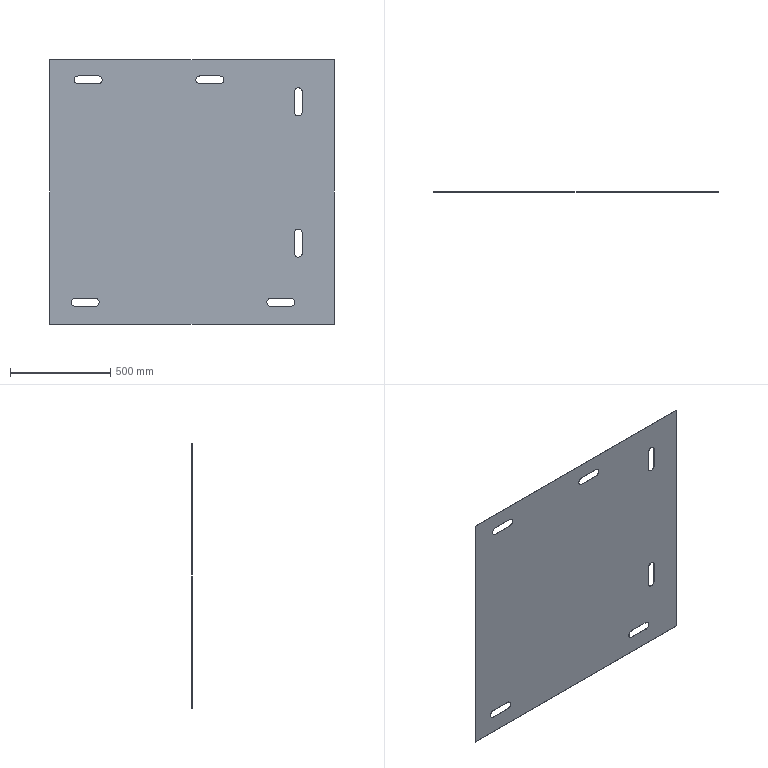Part | NX | features 切除-拉伸1 2 | 1 solid | 32 faces | box 1420 x 2 x 1320 mm | volume 3685720 mm3 | plane 18 | cylinder 14 | commonest cylinder face diameters 40 x14
STEP:
#1=CARTESIAN_POINT('',(622.78,-600.,-93.003));
#2=VERTEX_POINT('',#1);
#3=CARTESIAN_POINT('',(722.78,-600.,-93.003));
#4=VERTEX_POINT('',#3);
#5=CARTESIAN_POINT('',(622.78,-600.,-93.003));
#6=DIRECTION('',(1.,0.,0.));
#7=VECTOR('',#6,1000.);
#8=LINE('',#5,#7);
#9=EDGE_CURVE('',#2,#4,#8,.T.);
#10=ORIENTED_EDGE('',*,*,#9,.T.);
#11=CARTESIAN_POINT('',(722.78,-602.,-93.003));
#12=VERTEX_POINT('',#11);
#13=CARTESIAN_POINT('',(722.78,-602.,-93.003));
#14=DIRECTION('',(0.,1.,0.));
#15=VECTOR('',#14,1000.);
#16=LINE('',#13,#15);
#17=EDGE_CURVE('',#12,#4,#16,.T.);
#18=ORIENTED_EDGE('',*,*,#17,.F.);
#19=CARTESIAN_POINT('',(622.78,-602.,-93.003));
#20=VERTEX_POINT('',#19);
#21=CARTESIAN_POINT('',(622.78,-602.,-93.003));
#22=DIRECTION('',(1.,0.,0.));
#23=VECTOR('',#22,1000.);
#24=LINE('',#21,#23);
#25=EDGE_CURVE('',#20,#12,#24,.T.);
#26=ORIENTED_EDGE('',*,*,#25,.F.);
#27=CARTESIAN_POINT('',(622.78,-602.,-93.003));
#28=DIRECTION('',(0.,1.,0.));
#29=VECTOR('',#28,1000.);
#30=LINE('',#27,#29);
#31=EDGE_CURVE('',#20,#2,#30,.T.);
#32=ORIENTED_EDGE('',*,*,#31,.T.);
#33=EDGE_LOOP('',(#10,#18,#26,#32));
#34=FACE_BOUND('',#33,.T.);
#35=CARTESIAN_POINT('',(622.78,-602.,-93.003));
#36=DIRECTION('',(0.,0.,1.));
#37=DIRECTION('',(1.,0.,0.));
#38=AXIS2_PLACEMENT_3D('',#35,#36,#37);
#39=PLANE('',#38);
#40=ADVANCED_FACE('',(#34),#39,.F.);
#41=CARTESIAN_POINT('',(722.78,-600.,-133.003));
#42=VERTEX_POINT('',#41);
#43=CARTESIAN_POINT('',(722.78,-600.,-113.003));
#44=DIRECTION('',(0.,1.,0.));
#45=DIRECTION('',(0.,0.,1.));
#46=AXIS2_PLACEMENT_3D('',#43,#44,#45);
#47=CIRCLE('',#46,20.);
#48=EDGE_CURVE('',#4,#42,#47,.T.);
#49=ORIENTED_EDGE('',*,*,#48,.T.);
#50=CARTESIAN_POINT('',(722.78,-602.,-133.003));
#51=VERTEX_POINT('',#50);
#52=CARTESIAN_POINT('',(722.78,-602.,-133.003));
#53=DIRECTION('',(0.,1.,0.));
#54=VECTOR('',#53,1000.);
#55=LINE('',#52,#54);
#56=EDGE_CURVE('',#51,#42,#55,.T.);
#57=ORIENTED_EDGE('',*,*,#56,.F.);
#58=CARTESIAN_POINT('',(722.78,-602.,-113.003));
#59=DIRECTION('',(0.,1.,0.));
#60=DIRECTION('',(0.,0.,1.));
#61=AXIS2_PLACEMENT_3D('',#58,#59,#60);
#62=CIRCLE('',#61,20.);
#63=EDGE_CURVE('',#12,#51,#62,.T.);
#64=ORIENTED_EDGE('',*,*,#63,.F.);
#65=ORIENTED_EDGE('',*,*,#17,.T.);
#66=EDGE_LOOP('',(#49,#57,#64,#65));
#67=FACE_BOUND('',#66,.T.);
#68=CARTESIAN_POINT('',(722.78,-602.,-113.003));
#69=DIRECTION('',(0.,1.,0.));
#70=DIRECTION('',(0.,0.,1.));
#71=AXIS2_PLACEMENT_3D('',#68,#69,#70);
#72=CYLINDRICAL_SURFACE('',#71,20.);
#73=ADVANCED_FACE('',(#67),#72,.F.);
#74=CARTESIAN_POINT('',(622.78,-600.,-133.003));
#75=VERTEX_POINT('',#74);
#76=CARTESIAN_POINT('',(622.78,-600.,-133.003));
#77=DIRECTION('',(-1.,0.,0.));
#78=VECTOR('',#77,1000.);
#79=LINE('',#76,#78);
#80=EDGE_CURVE('',#42,#75,#79,.T.);
#81=ORIENTED_EDGE('',*,*,#80,.T.);
#82=CARTESIAN_POINT('',(622.78,-602.,-133.003));
#83=VERTEX_POINT('',#82);
#84=CARTESIAN_POINT('',(622.78,-602.,-133.003));
#85=DIRECTION('',(0.,1.,0.));
#86=VECTOR('',#85,1000.);
#87=LINE('',#84,#86);
#88=EDGE_CURVE('',#83,#75,#87,.T.);
#89=ORIENTED_EDGE('',*,*,#88,.F.);
#90=CARTESIAN_POINT('',(622.78,-602.,-133.003));
#91=DIRECTION('',(-1.,0.,0.));
#92=VECTOR('',#91,1000.);
#93=LINE('',#90,#92);
#94=EDGE_CURVE('',#51,#83,#93,.T.);
#95=ORIENTED_EDGE('',*,*,#94,.F.);
#96=ORIENTED_EDGE('',*,*,#56,.T.);
#97=EDGE_LOOP('',(#81,#89,#95,#96));
#98=FACE_BOUND('',#97,.T.);
#99=CARTESIAN_POINT('',(622.78,-602.,-133.003));
#100=DIRECTION('',(0.,0.,-1.));
#101=DIRECTION('',(-1.,0.,0.));
#102=AXIS2_PLACEMENT_3D('',#99,#100,#101);
#103=PLANE('',#102);
#104=ADVANCED_FACE('',(#98),#103,.F.);
#105=CARTESIAN_POINT('',(622.78,-600.,-113.003));
#106=DIRECTION('',(0.,1.,0.));
#107=DIRECTION('',(0.,0.,1.));
#108=AXIS2_PLACEMENT_3D('',#105,#106,#107);
#109=CIRCLE('',#108,20.);
#110=EDGE_CURVE('',#75,#2,#109,.T.);
#111=ORIENTED_EDGE('',*,*,#110,.T.);
#112=ORIENTED_EDGE('',*,*,#31,.F.);
#113=CARTESIAN_POINT('',(622.78,-602.,-113.003));
#114=DIRECTION('',(0.,1.,0.));
#115=DIRECTION('',(0.,0.,1.));
#116=AXIS2_PLACEMENT_3D('',#113,#114,#115);
#117=CIRCLE('',#116,20.);
#118=EDGE_CURVE('',#83,#20,#117,.T.);
#119=ORIENTED_EDGE('',*,*,#118,.F.);
#120=ORIENTED_EDGE('',*,*,#88,.T.);
#121=EDGE_LOOP('',(#111,#112,#119,#120));
#122=FACE_BOUND('',#121,.T.);
#123=CARTESIAN_POINT('',(622.78,-602.,-113.003));
#124=DIRECTION('',(0.,1.,0.));
#125=DIRECTION('',(0.,0.,1.));
#126=AXIS2_PLACEMENT_3D('',#123,#124,#125);
#127=CYLINDRICAL_SURFACE('',#126,20.);
#128=ADVANCED_FACE('',(#122),#127,.F.);
#129=CARTESIAN_POINT('',(-0.6402,-600.,-1204.113));
#130=VERTEX_POINT('',#129);
#131=CARTESIAN_POINT('',(99.36,-600.,-1204.113));
#132=VERTEX_POINT('',#131);
#133=CARTESIAN_POINT('',(-0.6402,-600.,-1204.113));
#134=DIRECTION('',(1.,0.,0.));
#135=VECTOR('',#134,1000.);
#136=LINE('',#133,#135);
#137=EDGE_CURVE('',#130,#132,#136,.T.);
#138=ORIENTED_EDGE('',*,*,#137,.T.);
#139=CARTESIAN_POINT('',(99.36,-602.,-1204.113));
#140=VERTEX_POINT('',#139);
#141=CARTESIAN_POINT('',(99.36,-602.,-1204.113));
#142=DIRECTION('',(0.,1.,0.));
#143=VECTOR('',#142,1000.);
#144=LINE('',#141,#143);
#145=EDGE_CURVE('',#140,#132,#144,.T.);
#146=ORIENTED_EDGE('',*,*,#145,.F.);
#147=CARTESIAN_POINT('',(-0.6402,-602.,-1204.113));
#148=VERTEX_POINT('',#147);
#149=CARTESIAN_POINT('',(-0.6402,-602.,-1204.113));
#150=DIRECTION('',(1.,0.,0.));
#151=VECTOR('',#150,1000.);
#152=LINE('',#149,#151);
#153=EDGE_CURVE('',#148,#140,#152,.T.);
#154=ORIENTED_EDGE('',*,*,#153,.F.);
#155=CARTESIAN_POINT('',(-0.6402,-602.,-1204.113));
#156=DIRECTION('',(0.,1.,0.));
#157=VECTOR('',#156,1000.);
#158=LINE('',#155,#157);
#159=EDGE_CURVE('',#148,#130,#158,.T.);
#160=ORIENTED_EDGE('',*,*,#159,.T.);
#161=EDGE_LOOP('',(#138,#146,#154,#160));
#162=FACE_BOUND('',#161,.T.);
#163=CARTESIAN_POINT('',(-0.6402,-602.,-1204.113));
#164=DIRECTION('',(0.,0.,1.));
#165=DIRECTION('',(1.,0.,0.));
#166=AXIS2_PLACEMENT_3D('',#163,#164,#165);
#167=PLANE('',#166);
#168=ADVANCED_FACE('',(#162),#167,.F.);
#169=CARTESIAN_POINT('',(99.36,-600.,-1244.113));
#170=VERTEX_POINT('',#169);
#171=CARTESIAN_POINT('',(99.36,-600.,-1224.113));
#172=DIRECTION('',(0.,1.,0.));
#173=DIRECTION('',(0.,0.,1.));
#174=AXIS2_PLACEMENT_3D('',#171,#172,#173);
#175=CIRCLE('',#174,20.);
#176=EDGE_CURVE('',#132,#170,#175,.T.);
#177=ORIENTED_EDGE('',*,*,#176,.T.);
#178=CARTESIAN_POINT('',(99.36,-602.,-1244.113));
#179=VERTEX_POINT('',#178);
#180=CARTESIAN_POINT('',(99.36,-602.,-1244.113));
#181=DIRECTION('',(0.,1.,0.));
#182=VECTOR('',#181,1000.);
#183=LINE('',#180,#182);
#184=EDGE_CURVE('',#179,#170,#183,.T.);
#185=ORIENTED_EDGE('',*,*,#184,.F.);
#186=CARTESIAN_POINT('',(99.36,-602.,-1224.113));
#187=DIRECTION('',(0.,1.,0.));
#188=DIRECTION('',(0.,0.,1.));
#189=AXIS2_PLACEMENT_3D('',#186,#187,#188);
#190=CIRCLE('',#189,20.);
#191=EDGE_CURVE('',#140,#179,#190,.T.);
#192=ORIENTED_EDGE('',*,*,#191,.F.);
#193=ORIENTED_EDGE('',*,*,#145,.T.);
#194=EDGE_LOOP('',(#177,#185,#192,#193));
#195=FACE_BOUND('',#194,.T.);
#196=CARTESIAN_POINT('',(99.36,-602.,-1224.113));
#197=DIRECTION('',(0.,1.,0.));
#198=DIRECTION('',(0.,0.,1.));
#199=AXIS2_PLACEMENT_3D('',#196,#197,#198);
#200=CYLINDRICAL_SURFACE('',#199,20.);
#201=ADVANCED_FACE('',(#195),#200,.F.);
#202=CARTESIAN_POINT('',(-0.6402,-600.,-1244.113));
#203=VERTEX_POINT('',#202);
#204=CARTESIAN_POINT('',(-0.6402,-600.,-1244.113));
#205=DIRECTION('',(-1.,0.,0.));
#206=VECTOR('',#205,1000.);
#207=LINE('',#204,#206);
#208=EDGE_CURVE('',#170,#203,#207,.T.);
#209=ORIENTED_EDGE('',*,*,#208,.T.);
#210=CARTESIAN_POINT('',(-0.6402,-602.,-1244.113));
#211=VERTEX_POINT('',#210);
#212=CARTESIAN_POINT('',(-0.6402,-602.,-1244.113));
#213=DIRECTION('',(0.,1.,0.));
#214=VECTOR('',#213,1000.);
#215=LINE('',#212,#214);
#216=EDGE_CURVE('',#211,#203,#215,.T.);
#217=ORIENTED_EDGE('',*,*,#216,.F.);
#218=CARTESIAN_POINT('',(-0.6402,-602.,-1244.113));
#219=DIRECTION('',(-1.,0.,0.));
#220=VECTOR('',#219,1000.);
#221=LINE('',#218,#220);
#222=EDGE_CURVE('',#179,#211,#221,.T.);
#223=ORIENTED_EDGE('',*,*,#222,.F.);
#224=ORIENTED_EDGE('',*,*,#184,.T.);
#225=EDGE_LOOP('',(#209,#217,#223,#224));
#226=FACE_BOUND('',#225,.T.);
#227=CARTESIAN_POINT('',(-0.6402,-602.,-1244.113));
#228=DIRECTION('',(0.,0.,-1.));
#229=DIRECTION('',(-1.,0.,0.));
#230=AXIS2_PLACEMENT_3D('',#227,#228,#229);
#231=PLANE('',#230);
#232=ADVANCED_FACE('',(#226),#231,.F.);
#233=CARTESIAN_POINT('',(-0.6402,-600.,-1224.113));
#234=DIRECTION('',(0.,1.,0.));
#235=DIRECTION('',(0.,0.,1.));
#236=AXIS2_PLACEMENT_3D('',#233,#234,#235);
#237=CIRCLE('',#236,20.);
#238=EDGE_CURVE('',#203,#130,#237,.T.);
#239=ORIENTED_EDGE('',*,*,#238,.T.);
#240=ORIENTED_EDGE('',*,*,#159,.F.);
#241=CARTESIAN_POINT('',(-0.6402,-602.,-1224.113));
#242=DIRECTION('',(0.,1.,0.));
#243=DIRECTION('',(0.,0.,1.));
#244=AXIS2_PLACEMENT_3D('',#241,#242,#243);
#245=CIRCLE('',#244,20.);
#246=EDGE_CURVE('',#211,#148,#245,.T.);
#247=ORIENTED_EDGE('',*,*,#246,.F.);
#248=ORIENTED_EDGE('',*,*,#216,.T.);
#249=EDGE_LOOP('',(#239,#240,#247,#248));
#250=FACE_BOUND('',#249,.T.);
#251=CARTESIAN_POINT('',(-0.6402,-602.,-1224.113));
#252=DIRECTION('',(0.,1.,0.));
#253=DIRECTION('',(0.,0.,1.));
#254=AXIS2_PLACEMENT_3D('',#251,#252,#253);
#255=CYLINDRICAL_SURFACE('',#254,20.);
#256=ADVANCED_FACE('',(#250),#255,.F.);
#257=CARTESIAN_POINT('',(976.615,-600.,-1204.113));
#258=VERTEX_POINT('',#257);
#259=CARTESIAN_POINT('',(1076.615,-600.,-1204.113));
#260=VERTEX_POINT('',#259);
#261=CARTESIAN_POINT('',(976.615,-600.,-1204.113));
#262=DIRECTION('',(1.,0.,0.));
#263=VECTOR('',#262,1000.);
#264=LINE('',#261,#263);
#265=EDGE_CURVE('',#258,#260,#264,.T.);
#266=ORIENTED_EDGE('',*,*,#265,.T.);
#267=CARTESIAN_POINT('',(1076.615,-602.,-1204.113));
#268=VERTEX_POINT('',#267);
#269=CARTESIAN_POINT('',(1076.615,-602.,-1204.113));
#270=DIRECTION('',(0.,1.,0.));
#271=VECTOR('',#270,1000.);
#272=LINE('',#269,#271);
#273=EDGE_CURVE('',#268,#260,#272,.T.);
#274=ORIENTED_EDGE('',*,*,#273,.F.);
#275=CARTESIAN_POINT('',(976.615,-602.,-1204.113));
#276=VERTEX_POINT('',#275);
#277=CARTESIAN_POINT('',(976.615,-602.,-1204.113));
#278=DIRECTION('',(1.,0.,0.));
#279=VECTOR('',#278,1000.);
#280=LINE('',#277,#279);
#281=EDGE_CURVE('',#276,#268,#280,.T.);
#282=ORIENTED_EDGE('',*,*,#281,.F.);
#283=CARTESIAN_POINT('',(976.615,-602.,-1204.113));
#284=DIRECTION('',(0.,1.,0.));
#285=VECTOR('',#284,1000.);
#286=LINE('',#283,#285);
#287=EDGE_CURVE('',#276,#258,#286,.T.);
#288=ORIENTED_EDGE('',*,*,#287,.T.);
#289=EDGE_LOOP('',(#266,#274,#282,#288));
#290=FACE_BOUND('',#289,.T.);
#291=CARTESIAN_POINT('',(976.615,-602.,-1204.113));
#292=DIRECTION('',(0.,0.,1.));
#293=DIRECTION('',(1.,0.,0.));
#294=AXIS2_PLACEMENT_3D('',#291,#292,#293);
#295=PLANE('',#294);
#296=ADVANCED_FACE('',(#290),#295,.F.);
#297=CARTESIAN_POINT('',(1076.615,-600.,-1244.113));
#298=VERTEX_POINT('',#297);
#299=CARTESIAN_POINT('',(1076.615,-600.,-1224.113));
#300=DIRECTION('',(0.,1.,0.));
#301=DIRECTION('',(0.,0.,1.));
#302=AXIS2_PLACEMENT_3D('',#299,#300,#301);
#303=CIRCLE('',#302,20.);
#304=EDGE_CURVE('',#260,#298,#303,.T.);
#305=ORIENTED_EDGE('',*,*,#304,.T.);
#306=CARTESIAN_POINT('',(1076.615,-602.,-1244.113));
#307=VERTEX_POINT('',#306);
#308=CARTESIAN_POINT('',(1076.615,-602.,-1244.113));
#309=DIRECTION('',(0.,1.,0.));
#310=VECTOR('',#309,1000.);
#311=LINE('',#308,#310);
#312=EDGE_CURVE('',#307,#298,#311,.T.);
#313=ORIENTED_EDGE('',*,*,#312,.F.);
#314=CARTESIAN_POINT('',(1076.615,-602.,-1224.113));
#315=DIRECTION('',(0.,1.,0.));
#316=DIRECTION('',(0.,0.,1.));
#317=AXIS2_PLACEMENT_3D('',#314,#315,#316);
#318=CIRCLE('',#317,20.);
#319=EDGE_CURVE('',#268,#307,#318,.T.);
#320=ORIENTED_EDGE('',*,*,#319,.F.);
#321=ORIENTED_EDGE('',*,*,#273,.T.);
#322=EDGE_LOOP('',(#305,#313,#320,#321));
#323=FACE_BOUND('',#322,.T.);
#324=CARTESIAN_POINT('',(1076.615,-602.,-1224.113));
#325=DIRECTION('',(0.,1.,0.));
#326=DIRECTION('',(0.,0.,1.));
#327=AXIS2_PLACEMENT_3D('',#324,#325,#326);
#328=CYLINDRICAL_SURFACE('',#327,20.);
#329=ADVANCED_FACE('',(#323),#328,.F.);
#330=CARTESIAN_POINT('',(976.615,-600.,-1244.113));
#331=VERTEX_POINT('',#330);
#332=CARTESIAN_POINT('',(976.615,-600.,-1244.113));
#333=DIRECTION('',(-1.,0.,0.));
#334=VECTOR('',#333,1000.);
#335=LINE('',#332,#334);
#336=EDGE_CURVE('',#298,#331,#335,.T.);
#337=ORIENTED_EDGE('',*,*,#336,.T.);
#338=CARTESIAN_POINT('',(976.615,-602.,-1244.113));
#339=VERTEX_POINT('',#338);
#340=CARTESIAN_POINT('',(976.615,-602.,-1244.113));
#341=DIRECTION('',(0.,1.,0.));
#342=VECTOR('',#341,1000.);
#343=LINE('',#340,#342);
#344=EDGE_CURVE('',#339,#331,#343,.T.);
#345=ORIENTED_EDGE('',*,*,#344,.F.);
#346=CARTESIAN_POINT('',(976.615,-602.,-1244.113));
#347=DIRECTION('',(-1.,0.,0.));
#348=VECTOR('',#347,1000.);
#349=LINE('',#346,#348);
#350=EDGE_CURVE('',#307,#339,#349,.T.);
#351=ORIENTED_EDGE('',*,*,#350,.F.);
#352=ORIENTED_EDGE('',*,*,#312,.T.);
#353=EDGE_LOOP('',(#337,#345,#351,#352));
#354=FACE_BOUND('',#353,.T.);
#355=CARTESIAN_POINT('',(976.615,-602.,-1244.113));
#356=DIRECTION('',(0.,0.,-1.));
#357=DIRECTION('',(-1.,0.,0.));
#358=AXIS2_PLACEMENT_3D('',#355,#356,#357);
#359=PLANE('',#358);
#360=ADVANCED_FACE('',(#354),#359,.F.);
#361=CARTESIAN_POINT('',(976.615,-600.,-1224.113));
#362=DIRECTION('',(0.,1.,0.));
#363=DIRECTION('',(0.,0.,1.));
#364=AXIS2_PLACEMENT_3D('',#361,#362,#363);
#365=CIRCLE('',#364,20.);
#366=EDGE_CURVE('',#331,#258,#365,.T.);
#367=ORIENTED_EDGE('',*,*,#366,.T.);
#368=ORIENTED_EDGE('',*,*,#287,.F.);
#369=CARTESIAN_POINT('',(976.615,-602.,-1224.113));
#370=DIRECTION('',(0.,1.,0.));
#371=DIRECTION('',(0.,0.,1.));
#372=AXIS2_PLACEMENT_3D('',#369,#370,#371);
#373=CIRCLE('',#372,20.);
#374=EDGE_CURVE('',#339,#276,#373,.T.);
#375=ORIENTED_EDGE('',*,*,#374,.F.);
#376=ORIENTED_EDGE('',*,*,#344,.T.);
#377=EDGE_LOOP('',(#367,#368,#375,#376));
#378=FACE_BOUND('',#377,.T.);
#379=CARTESIAN_POINT('',(976.615,-602.,-1224.113));
#380=DIRECTION('',(0.,1.,0.));
#381=DIRECTION('',(0.,0.,1.));
#382=AXIS2_PLACEMENT_3D('',#379,#380,#381);
#383=CYLINDRICAL_SURFACE('',#382,20.);
#384=ADVANCED_FACE('',(#378),#383,.F.);
#385=CARTESIAN_POINT('',(1133.771,-600.,-878.167));
#386=VERTEX_POINT('',#385);
#387=CARTESIAN_POINT('',(1133.771,-600.,-978.167));
#388=VERTEX_POINT('',#387);
#389=CARTESIAN_POINT('',(1133.771,-600.,-878.167));
#390=DIRECTION('',(0.,0.,-1.));
#391=VECTOR('',#390,1000.);
#392=LINE('',#389,#391);
#393=EDGE_CURVE('',#386,#388,#392,.T.);
#394=ORIENTED_EDGE('',*,*,#393,.T.);
#395=CARTESIAN_POINT('',(1133.771,-602.,-978.167));
#396=VERTEX_POINT('',#395);
#397=CARTESIAN_POINT('',(1133.771,-602.,-978.167));
#398=DIRECTION('',(0.,1.,0.));
#399=VECTOR('',#398,1000.);
#400=LINE('',#397,#399);
#401=EDGE_CURVE('',#396,#388,#400,.T.);
#402=ORIENTED_EDGE('',*,*,#401,.F.);
#403=CARTESIAN_POINT('',(1133.771,-602.,-878.167));
#404=VERTEX_POINT('',#403);
#405=CARTESIAN_POINT('',(1133.771,-602.,-878.167));
#406=DIRECTION('',(0.,0.,-1.));
#407=VECTOR('',#406,1000.);
#408=LINE('',#405,#407);
#409=EDGE_CURVE('',#404,#396,#408,.T.);
#410=ORIENTED_EDGE('',*,*,#409,.F.);
#411=CARTESIAN_POINT('',(1133.771,-602.,-878.167));
#412=DIRECTION('',(0.,1.,0.));
#413=VECTOR('',#412,1000.);
#414=LINE('',#411,#413);
#415=EDGE_CURVE('',#404,#386,#414,.T.);
#416=ORIENTED_EDGE('',*,*,#415,.T.);
#417=EDGE_LOOP('',(#394,#402,#410,#416));
#418=FACE_BOUND('',#417,.T.);
#419=CARTESIAN_POINT('',(1133.771,-602.,-878.167));
#420=DIRECTION('',(1.,0.,0.));
#421=DIRECTION('',(0.,0.,-1.));
#422=AXIS2_PLACEMENT_3D('',#419,#420,#421);
#423=PLANE('',#422);
#424=ADVANCED_FACE('',(#418),#423,.F.);
#425=CARTESIAN_POINT('',(1093.771,-600.,-978.167));
#426=VERTEX_POINT('',#425);
#427=CARTESIAN_POINT('',(1113.771,-600.,-978.167));
#428=DIRECTION('',(0.,1.,0.));
#429=DIRECTION('',(0.,0.,1.));
#430=AXIS2_PLACEMENT_3D('',#427,#428,#429);
#431=CIRCLE('',#430,20.);
#432=EDGE_CURVE('',#388,#426,#431,.T.);
#433=ORIENTED_EDGE('',*,*,#432,.T.);
#434=CARTESIAN_POINT('',(1093.771,-602.,-978.167));
#435=VERTEX_POINT('',#434);
#436=CARTESIAN_POINT('',(1093.771,-602.,-978.167));
#437=DIRECTION('',(0.,1.,0.));
#438=VECTOR('',#437,1000.);
#439=LINE('',#436,#438);
#440=EDGE_CURVE('',#435,#426,#439,.T.);
#441=ORIENTED_EDGE('',*,*,#440,.F.);
#442=CARTESIAN_POINT('',(1113.771,-602.,-978.167));
#443=DIRECTION('',(0.,1.,0.));
#444=DIRECTION('',(0.,0.,1.));
#445=AXIS2_PLACEMENT_3D('',#442,#443,#444);
#446=CIRCLE('',#445,20.);
#447=EDGE_CURVE('',#396,#435,#446,.T.);
#448=ORIENTED_EDGE('',*,*,#447,.F.);
#449=ORIENTED_EDGE('',*,*,#401,.T.);
#450=EDGE_LOOP('',(#433,#441,#448,#449));
#451=FACE_BOUND('',#450,.T.);
#452=CARTESIAN_POINT('',(1113.771,-602.,-978.167));
#453=DIRECTION('',(0.,1.,0.));
#454=DIRECTION('',(0.,0.,1.));
#455=AXIS2_PLACEMENT_3D('',#452,#453,#454);
#456=CYLINDRICAL_SURFACE('',#455,20.);
#457=ADVANCED_FACE('',(#451),#456,.F.);
#458=CARTESIAN_POINT('',(1093.771,-600.,-878.167));
#459=VERTEX_POINT('',#458);
#460=CARTESIAN_POINT('',(1093.771,-600.,-878.167));
#461=DIRECTION('',(0.,0.,1.));
#462=VECTOR('',#461,1000.);
#463=LINE('',#460,#462);
#464=EDGE_CURVE('',#426,#459,#463,.T.);
#465=ORIENTED_EDGE('',*,*,#464,.T.);
#466=CARTESIAN_POINT('',(1093.771,-602.,-878.167));
#467=VERTEX_POINT('',#466);
#468=CARTESIAN_POINT('',(1093.771,-602.,-878.167));
#469=DIRECTION('',(0.,1.,0.));
#470=VECTOR('',#469,1000.);
#471=LINE('',#468,#470);
#472=EDGE_CURVE('',#467,#459,#471,.T.);
#473=ORIENTED_EDGE('',*,*,#472,.F.);
#474=CARTESIAN_POINT('',(1093.771,-602.,-878.167));
#475=DIRECTION('',(0.,0.,1.));
#476=VECTOR('',#475,1000.);
#477=LINE('',#474,#476);
#478=EDGE_CURVE('',#435,#467,#477,.T.);
#479=ORIENTED_EDGE('',*,*,#478,.F.);
#480=ORIENTED_EDGE('',*,*,#440,.T.);
#481=EDGE_LOOP('',(#465,#473,#479,#480));
#482=FACE_BOUND('',#481,.T.);
#483=CARTESIAN_POINT('',(1093.771,-602.,-878.167));
#484=DIRECTION('',(-1.,0.,0.));
#485=DIRECTION('',(0.,0.,1.));
#486=AXIS2_PLACEMENT_3D('',#483,#484,#485);
#487=PLANE('',#486);
#488=ADVANCED_FACE('',(#482),#487,.F.);
#489=CARTESIAN_POINT('',(1113.771,-602.,-858.167));
#490=VERTEX_POINT('',#489);
#491=CARTESIAN_POINT('',(1113.771,-600.,-858.167));
#492=VERTEX_POINT('',#491);
#493=CARTESIAN_POINT('',(1113.771,-602.,-858.167));
#494=DIRECTION('',(0.,1.,0.));
#495=VECTOR('',#494,1000.);
#496=LINE('',#493,#495);
#497=EDGE_CURVE('',#490,#492,#496,.T.);
#498=ORIENTED_EDGE('',*,*,#497,.F.);
#499=CARTESIAN_POINT('',(1113.771,-602.,-878.167));
#500=DIRECTION('',(0.,1.,0.));
#501=DIRECTION('',(0.,0.,1.));
#502=AXIS2_PLACEMENT_3D('',#499,#500,#501);
#503=CIRCLE('',#502,20.);
#504=EDGE_CURVE('',#467,#490,#503,.T.);
#505=ORIENTED_EDGE('',*,*,#504,.F.);
#506=ORIENTED_EDGE('',*,*,#472,.T.);
#507=CARTESIAN_POINT('',(1113.771,-600.,-878.167));
#508=DIRECTION('',(0.,1.,0.));
#509=DIRECTION('',(0.,0.,1.));
#510=AXIS2_PLACEMENT_3D('',#507,#508,#509);
#511=CIRCLE('',#510,20.);
#512=EDGE_CURVE('',#459,#492,#511,.T.);
#513=ORIENTED_EDGE('',*,*,#512,.T.);
#514=EDGE_LOOP('',(#498,#505,#506,#513));
#515=FACE_BOUND('',#514,.T.);
#516=CARTESIAN_POINT('',(1113.771,-602.,-878.167));
#517=DIRECTION('',(0.,1.,0.));
#518=DIRECTION('',(0.,0.,1.));
#519=AXIS2_PLACEMENT_3D('',#516,#517,#518);
#520=CYLINDRICAL_SURFACE('',#519,20.);
#521=ADVANCED_FACE('',(#515),#520,.F.);
#522=CARTESIAN_POINT('',(1133.771,-600.,-172.209));
#523=VERTEX_POINT('',#522);
#524=CARTESIAN_POINT('',(1133.771,-600.,-272.209));
#525=VERTEX_POINT('',#524);
#526=CARTESIAN_POINT('',(1133.771,-600.,-172.209));
#527=DIRECTION('',(0.,0.,-1.));
#528=VECTOR('',#527,1000.);
#529=LINE('',#526,#528);
#530=EDGE_CURVE('',#523,#525,#529,.T.);
#531=ORIENTED_EDGE('',*,*,#530,.T.);
#532=CARTESIAN_POINT('',(1133.771,-602.,-272.209));
#533=VERTEX_POINT('',#532);
#534=CARTESIAN_POINT('',(1133.771,-602.,-272.209));
#535=DIRECTION('',(0.,1.,0.));
#536=VECTOR('',#535,1000.);
#537=LINE('',#534,#536);
#538=EDGE_CURVE('',#533,#525,#537,.T.);
#539=ORIENTED_EDGE('',*,*,#538,.F.);
#540=CARTESIAN_POINT('',(1133.771,-602.,-172.209));
#541=VERTEX_POINT('',#540);
#542=CARTESIAN_POINT('',(1133.771,-602.,-172.209));
#543=DIRECTION('',(0.,0.,-1.));
#544=VECTOR('',#543,1000.);
#545=LINE('',#542,#544);
#546=EDGE_CURVE('',#541,#533,#545,.T.);
#547=ORIENTED_EDGE('',*,*,#546,.F.);
#548=CARTESIAN_POINT('',(1133.771,-602.,-172.209));
#549=DIRECTION('',(0.,1.,0.));
#550=VECTOR('',#549,1000.);
#551=LINE('',#548,#550);
#552=EDGE_CURVE('',#541,#523,#551,.T.);
#553=ORIENTED_EDGE('',*,*,#552,.T.);
#554=EDGE_LOOP('',(#531,#539,#547,#553));
#555=FACE_BOUND('',#554,.T.);
#556=CARTESIAN_POINT('',(1133.771,-602.,-172.209));
#557=DIRECTION('',(1.,0.,0.));
#558=DIRECTION('',(0.,0.,-1.));
#559=AXIS2_PLACEMENT_3D('',#556,#557,#558);
#560=PLANE('',#559);
#561=ADVANCED_FACE('',(#555),#560,.F.);
#562=CARTESIAN_POINT('',(1093.771,-600.,-272.209));
#563=VERTEX_POINT('',#562);
#564=CARTESIAN_POINT('',(1113.771,-600.,-272.209));
#565=DIRECTION('',(0.,1.,0.));
#566=DIRECTION('',(0.,0.,1.));
#567=AXIS2_PLACEMENT_3D('',#564,#565,#566);
#568=CIRCLE('',#567,20.);
#569=EDGE_CURVE('',#525,#563,#568,.T.);
#570=ORIENTED_EDGE('',*,*,#569,.T.);
#571=CARTESIAN_POINT('',(1093.771,-602.,-272.209));
#572=VERTEX_POINT('',#571);
#573=CARTESIAN_POINT('',(1093.771,-602.,-272.209));
#574=DIRECTION('',(0.,1.,0.));
#575=VECTOR('',#574,1000.);
#576=LINE('',#573,#575);
#577=EDGE_CURVE('',#572,#563,#576,.T.);
#578=ORIENTED_EDGE('',*,*,#577,.F.);
#579=CARTESIAN_POINT('',(1113.771,-602.,-272.209));
#580=DIRECTION('',(0.,1.,0.));
#581=DIRECTION('',(0.,0.,1.));
#582=AXIS2_PLACEMENT_3D('',#579,#580,#581);
#583=CIRCLE('',#582,20.);
#584=EDGE_CURVE('',#533,#572,#583,.T.);
#585=ORIENTED_EDGE('',*,*,#584,.F.);
#586=ORIENTED_EDGE('',*,*,#538,.T.);
#587=EDGE_LOOP('',(#570,#578,#585,#586));
#588=FACE_BOUND('',#587,.T.);
#589=CARTESIAN_POINT('',(1113.771,-602.,-272.209));
#590=DIRECTION('',(0.,1.,0.));
#591=DIRECTION('',(0.,0.,1.));
#592=AXIS2_PLACEMENT_3D('',#589,#590,#591);
#593=CYLINDRICAL_SURFACE('',#592,20.);
#594=ADVANCED_FACE('',(#588),#593,.F.);
#595=CARTESIAN_POINT('',(1093.771,-600.,-172.209));
#596=VERTEX_POINT('',#595);
#597=CARTESIAN_POINT('',(1093.771,-600.,-172.209));
#598=DIRECTION('',(0.,0.,1.));
#599=VECTOR('',#598,1000.);
#600=LINE('',#597,#599);
#601=EDGE_CURVE('',#563,#596,#600,.T.);
#602=ORIENTED_EDGE('',*,*,#601,.T.);
#603=CARTESIAN_POINT('',(1093.771,-602.,-172.209));
#604=VERTEX_POINT('',#603);
#605=CARTESIAN_POINT('',(1093.771,-602.,-172.209));
#606=DIRECTION('',(0.,1.,0.));
#607=VECTOR('',#606,1000.);
#608=LINE('',#605,#607);
#609=EDGE_CURVE('',#604,#596,#608,.T.);
#610=ORIENTED_EDGE('',*,*,#609,.F.);
#611=CARTESIAN_POINT('',(1093.771,-602.,-172.209));
#612=DIRECTION('',(0.,0.,1.));
#613=VECTOR('',#612,1000.);
#614=LINE('',#611,#613);
#615=EDGE_CURVE('',#572,#604,#614,.T.);
#616=ORIENTED_EDGE('',*,*,#615,.F.);
#617=ORIENTED_EDGE('',*,*,#577,.T.);
#618=EDGE_LOOP('',(#602,#610,#616,#617));
#619=FACE_BOUND('',#618,.T.);
#620=CARTESIAN_POINT('',(1093.771,-602.,-172.209));
#621=DIRECTION('',(-1.,0.,0.));
#622=DIRECTION('',(0.,0.,1.));
#623=AXIS2_PLACEMENT_3D('',#620,#621,#622);
#624=PLANE('',#623);
#625=ADVANCED_FACE('',(#619),#624,.F.);
#626=CARTESIAN_POINT('',(1113.771,-602.,-152.209));
#627=VERTEX_POINT('',#626);
#628=CARTESIAN_POINT('',(1113.771,-600.,-152.209));
#629=VERTEX_POINT('',#628);
#630=CARTESIAN_POINT('',(1113.771,-602.,-152.209));
#631=DIRECTION('',(0.,1.,0.));
#632=VECTOR('',#631,1000.);
#633=LINE('',#630,#632);
#634=EDGE_CURVE('',#627,#629,#633,.T.);
#635=ORIENTED_EDGE('',*,*,#634,.F.);
#636=CARTESIAN_POINT('',(1113.771,-602.,-172.209));
#637=DIRECTION('',(0.,1.,0.));
#638=DIRECTION('',(0.,0.,1.));
#639=AXIS2_PLACEMENT_3D('',#636,#637,#638);
#640=CIRCLE('',#639,20.);
#641=EDGE_CURVE('',#604,#627,#640,.T.);
#642=ORIENTED_EDGE('',*,*,#641,.F.);
#643=ORIENTED_EDGE('',*,*,#609,.T.);
#644=CARTESIAN_POINT('',(1113.771,-600.,-172.209));
#645=DIRECTION('',(0.,1.,0.));
#646=DIRECTION('',(0.,0.,1.));
#647=AXIS2_PLACEMENT_3D('',#644,#645,#646);
#648=CIRCLE('',#647,20.);
#649=EDGE_CURVE('',#596,#629,#648,.T.);
#650=ORIENTED_EDGE('',*,*,#649,.T.);
#651=EDGE_LOOP('',(#635,#642,#643,#650));
#652=FACE_BOUND('',#651,.T.);
#653=CARTESIAN_POINT('',(1113.771,-602.,-172.209));
#654=DIRECTION('',(0.,1.,0.));
#655=DIRECTION('',(0.,0.,1.));
#656=AXIS2_PLACEMENT_3D('',#653,#654,#655);
#657=CYLINDRICAL_SURFACE('',#656,20.);
#658=ADVANCED_FACE('',(#652),#657,.F.);
#659=CARTESIAN_POINT('',(14.249,-600.,-93.003));
#660=VERTEX_POINT('',#659);
#661=CARTESIAN_POINT('',(114.249,-600.,-93.003));
#662=VERTEX_POINT('',#661);
#663=CARTESIAN_POINT('',(14.249,-600.,-93.003));
#664=DIRECTION('',(1.,0.,0.));
#665=VECTOR('',#664,1000.);
#666=LINE('',#663,#665);
#667=EDGE_CURVE('',#660,#662,#666,.T.);
#668=ORIENTED_EDGE('',*,*,#667,.T.);
#669=CARTESIAN_POINT('',(114.249,-602.,-93.003));
#670=VERTEX_POINT('',#669);
#671=CARTESIAN_POINT('',(114.249,-602.,-93.003));
#672=DIRECTION('',(0.,1.,0.));
#673=VECTOR('',#672,1000.);
#674=LINE('',#671,#673);
#675=EDGE_CURVE('',#670,#662,#674,.T.);
#676=ORIENTED_EDGE('',*,*,#675,.F.);
#677=CARTESIAN_POINT('',(14.249,-602.,-93.003));
#678=VERTEX_POINT('',#677);
#679=CARTESIAN_POINT('',(14.249,-602.,-93.003));
#680=DIRECTION('',(1.,0.,0.));
#681=VECTOR('',#680,1000.);
#682=LINE('',#679,#681);
#683=EDGE_CURVE('',#678,#670,#682,.T.);
#684=ORIENTED_EDGE('',*,*,#683,.F.);
#685=CARTESIAN_POINT('',(14.249,-602.,-93.003));
#686=DIRECTION('',(0.,1.,0.));
#687=VECTOR('',#686,1000.);
#688=LINE('',#685,#687);
#689=EDGE_CURVE('',#678,#660,#688,.T.);
#690=ORIENTED_EDGE('',*,*,#689,.T.);
#691=EDGE_LOOP('',(#668,#676,#684,#690));
#692=FACE_BOUND('',#691,.T.);
#693=CARTESIAN_POINT('',(14.249,-602.,-93.003));
#694=DIRECTION('',(0.,0.,1.));
#695=DIRECTION('',(1.,0.,0.));
#696=AXIS2_PLACEMENT_3D('',#693,#694,#695);
#697=PLANE('',#696);
#698=ADVANCED_FACE('',(#692),#697,.F.);
#699=CARTESIAN_POINT('',(114.249,-600.,-133.003));
#700=VERTEX_POINT('',#699);
#701=CARTESIAN_POINT('',(114.249,-600.,-113.003));
#702=DIRECTION('',(0.,1.,0.));
#703=DIRECTION('',(0.,0.,1.));
#704=AXIS2_PLACEMENT_3D('',#701,#702,#703);
#705=CIRCLE('',#704,20.);
#706=EDGE_CURVE('',#662,#700,#705,.T.);
#707=ORIENTED_EDGE('',*,*,#706,.T.);
#708=CARTESIAN_POINT('',(114.249,-602.,-133.003));
#709=VERTEX_POINT('',#708);
#710=CARTESIAN_POINT('',(114.249,-602.,-133.003));
#711=DIRECTION('',(0.,1.,0.));
#712=VECTOR('',#711,1000.);
#713=LINE('',#710,#712);
#714=EDGE_CURVE('',#709,#700,#713,.T.);
#715=ORIENTED_EDGE('',*,*,#714,.F.);
#716=CARTESIAN_POINT('',(114.249,-602.,-113.003));
#717=DIRECTION('',(0.,1.,0.));
#718=DIRECTION('',(0.,0.,1.));
#719=AXIS2_PLACEMENT_3D('',#716,#717,#718);
#720=CIRCLE('',#719,20.);
#721=EDGE_CURVE('',#670,#709,#720,.T.);
#722=ORIENTED_EDGE('',*,*,#721,.F.);
#723=ORIENTED_EDGE('',*,*,#675,.T.);
#724=EDGE_LOOP('',(#707,#715,#722,#723));
#725=FACE_BOUND('',#724,.T.);
#726=CARTESIAN_POINT('',(114.249,-602.,-113.003));
#727=DIRECTION('',(0.,1.,0.));
#728=DIRECTION('',(0.,0.,1.));
#729=AXIS2_PLACEMENT_3D('',#726,#727,#728);
#730=CYLINDRICAL_SURFACE('',#729,20.);
#731=ADVANCED_FACE('',(#725),#730,.F.);
#732=CARTESIAN_POINT('',(14.249,-600.,-133.003));
#733=VERTEX_POINT('',#732);
#734=CARTESIAN_POINT('',(14.249,-600.,-133.003));
#735=DIRECTION('',(-1.,0.,0.));
#736=VECTOR('',#735,1000.);
#737=LINE('',#734,#736);
#738=EDGE_CURVE('',#700,#733,#737,.T.);
#739=ORIENTED_EDGE('',*,*,#738,.T.);
#740=CARTESIAN_POINT('',(14.249,-602.,-133.003));
#741=VERTEX_POINT('',#740);
#742=CARTESIAN_POINT('',(14.249,-602.,-133.003));
#743=DIRECTION('',(0.,1.,0.));
#744=VECTOR('',#743,1000.);
#745=LINE('',#742,#744);
#746=EDGE_CURVE('',#741,#733,#745,.T.);
#747=ORIENTED_EDGE('',*,*,#746,.F.);
#748=CARTESIAN_POINT('',(14.249,-602.,-133.003));
#749=DIRECTION('',(-1.,0.,0.));
#750=VECTOR('',#749,1000.);
#751=LINE('',#748,#750);
#752=EDGE_CURVE('',#709,#741,#751,.T.);
#753=ORIENTED_EDGE('',*,*,#752,.F.);
#754=ORIENTED_EDGE('',*,*,#714,.T.);
#755=EDGE_LOOP('',(#739,#747,#753,#754));
#756=FACE_BOUND('',#755,.T.);
#757=CARTESIAN_POINT('',(14.249,-602.,-133.003));
#758=DIRECTION('',(0.,0.,-1.));
#759=DIRECTION('',(-1.,0.,0.));
#760=AXIS2_PLACEMENT_3D('',#757,#758,#759);
#761=PLANE('',#760);
#762=ADVANCED_FACE('',(#756),#761,.F.);
#763=CARTESIAN_POINT('',(14.249,-600.,-113.003));
#764=DIRECTION('',(0.,1.,0.));
#765=DIRECTION('',(0.,0.,1.));
#766=AXIS2_PLACEMENT_3D('',#763,#764,#765);
#767=CIRCLE('',#766,20.);
#768=EDGE_CURVE('',#733,#660,#767,.T.);
#769=ORIENTED_EDGE('',*,*,#768,.T.);
#770=ORIENTED_EDGE('',*,*,#689,.F.);
#771=CARTESIAN_POINT('',(14.249,-602.,-113.003));
#772=DIRECTION('',(0.,1.,0.));
#773=DIRECTION('',(0.,0.,1.));
#774=AXIS2_PLACEMENT_3D('',#771,#772,#773);
#775=CIRCLE('',#774,20.);
#776=EDGE_CURVE('',#741,#678,#775,.T.);
#777=ORIENTED_EDGE('',*,*,#776,.F.);
#778=ORIENTED_EDGE('',*,*,#746,.T.);
#779=EDGE_LOOP('',(#769,#770,#777,#778));
#780=FACE_BOUND('',#779,.T.);
#781=CARTESIAN_POINT('',(14.249,-602.,-113.003));
#782=DIRECTION('',(0.,1.,0.));
#783=DIRECTION('',(0.,0.,1.));
#784=AXIS2_PLACEMENT_3D('',#781,#782,#783);
#785=CYLINDRICAL_SURFACE('',#784,20.);
#786=ADVANCED_FACE('',(#780),#785,.F.);
#787=CARTESIAN_POINT('',(-127.,-600.,-12.985));
#788=VERTEX_POINT('',#787);
#789=CARTESIAN_POINT('',(-127.,-600.,-1332.985));
#790=VERTEX_POINT('',#789);
#791=CARTESIAN_POINT('',(-127.,-600.,-12.985));
#792=DIRECTION('',(0.,0.,-1.));
#793=VECTOR('',#792,1000.);
#794=LINE('',#791,#793);
#795=EDGE_CURVE('',#788,#790,#794,.T.);
#796=ORIENTED_EDGE('',*,*,#795,.F.);
#797=CARTESIAN_POINT('',(1293.,-600.,-12.985));
#798=VERTEX_POINT('',#797);
#799=CARTESIAN_POINT('',(-127.,-600.,-12.985));
#800=DIRECTION('',(-1.,0.,0.));
#801=VECTOR('',#800,1000.);
#802=LINE('',#799,#801);
#803=EDGE_CURVE('',#798,#788,#802,.T.);
#804=ORIENTED_EDGE('',*,*,#803,.F.);
#805=CARTESIAN_POINT('',(1293.,-600.,-1332.985));
#806=VERTEX_POINT('',#805);
#807=CARTESIAN_POINT('',(1293.,-600.,-12.985));
#808=DIRECTION('',(0.,0.,1.));
#809=VECTOR('',#808,1000.);
#810=LINE('',#807,#809);
#811=EDGE_CURVE('',#806,#798,#810,.T.);
#812=ORIENTED_EDGE('',*,*,#811,.F.);
#813=CARTESIAN_POINT('',(-127.,-600.,-1332.985));
#814=DIRECTION('',(1.,0.,0.));
#815=VECTOR('',#814,1000.);
#816=LINE('',#813,#815);
#817=EDGE_CURVE('',#790,#806,#816,.T.);
#818=ORIENTED_EDGE('',*,*,#817,.F.);
#819=EDGE_LOOP('',(#796,#804,#812,#818));
#820=FACE_BOUND('',#819,.T.);
#821=ORIENTED_EDGE('',*,*,#667,.F.);
#822=ORIENTED_EDGE('',*,*,#768,.F.);
#823=ORIENTED_EDGE('',*,*,#738,.F.);
#824=ORIENTED_EDGE('',*,*,#706,.F.);
#825=EDGE_LOOP('',(#821,#822,#823,#824));
#826=FACE_BOUND('',#825,.T.);
#827=ORIENTED_EDGE('',*,*,#530,.F.);
#828=CARTESIAN_POINT('',(1113.771,-600.,-172.209));
#829=DIRECTION('',(0.,1.,0.));
#830=DIRECTION('',(0.,0.,1.));
#831=AXIS2_PLACEMENT_3D('',#828,#829,#830);
#832=CIRCLE('',#831,20.);
#833=EDGE_CURVE('',#629,#523,#832,.T.);
#834=ORIENTED_EDGE('',*,*,#833,.F.);
#835=ORIENTED_EDGE('',*,*,#649,.F.);
#836=ORIENTED_EDGE('',*,*,#601,.F.);
#837=ORIENTED_EDGE('',*,*,#569,.F.);
#838=EDGE_LOOP('',(#827,#834,#835,#836,#837));
#839=FACE_BOUND('',#838,.T.);
#840=ORIENTED_EDGE('',*,*,#393,.F.);
#841=CARTESIAN_POINT('',(1113.771,-600.,-878.167));
#842=DIRECTION('',(0.,1.,0.));
#843=DIRECTION('',(0.,0.,1.));
#844=AXIS2_PLACEMENT_3D('',#841,#842,#843);
#845=CIRCLE('',#844,20.);
#846=EDGE_CURVE('',#492,#386,#845,.T.);
#847=ORIENTED_EDGE('',*,*,#846,.F.);
#848=ORIENTED_EDGE('',*,*,#512,.F.);
#849=ORIENTED_EDGE('',*,*,#464,.F.);
#850=ORIENTED_EDGE('',*,*,#432,.F.);
#851=EDGE_LOOP('',(#840,#847,#848,#849,#850));
#852=FACE_BOUND('',#851,.T.);
#853=ORIENTED_EDGE('',*,*,#265,.F.);
#854=ORIENTED_EDGE('',*,*,#366,.F.);
#855=ORIENTED_EDGE('',*,*,#336,.F.);
#856=ORIENTED_EDGE('',*,*,#304,.F.);
#857=EDGE_LOOP('',(#853,#854,#855,#856));
#858=FACE_BOUND('',#857,.T.);
#859=ORIENTED_EDGE('',*,*,#137,.F.);
#860=ORIENTED_EDGE('',*,*,#238,.F.);
#861=ORIENTED_EDGE('',*,*,#208,.F.);
#862=ORIENTED_EDGE('',*,*,#176,.F.);
#863=EDGE_LOOP('',(#859,#860,#861,#862));
#864=FACE_BOUND('',#863,.T.);
#865=ORIENTED_EDGE('',*,*,#9,.F.);
#866=ORIENTED_EDGE('',*,*,#110,.F.);
#867=ORIENTED_EDGE('',*,*,#80,.F.);
#868=ORIENTED_EDGE('',*,*,#48,.F.);
#869=EDGE_LOOP('',(#865,#866,#867,#868));
#870=FACE_BOUND('',#869,.T.);
#871=CARTESIAN_POINT('',(0.,-600.,0.));
#872=DIRECTION('',(0.,-1.,0.));
#873=DIRECTION('',(0.,0.,-1.));
#874=AXIS2_PLACEMENT_3D('',#871,#872,#873);
#875=PLANE('',#874);
#876=ADVANCED_FACE('',(#820,#826,#839,#852,#858,#864,#870),#875,.F.);
#877=CARTESIAN_POINT('',(-127.,-602.,-12.985));
#878=VERTEX_POINT('',#877);
#879=CARTESIAN_POINT('',(-127.,-602.,-1332.985));
#880=VERTEX_POINT('',#879);
#881=CARTESIAN_POINT('',(-127.,-602.,-12.985));
#882=DIRECTION('',(0.,0.,-1.));
#883=VECTOR('',#882,1000.);
#884=LINE('',#881,#883);
#885=EDGE_CURVE('',#878,#880,#884,.T.);
#886=ORIENTED_EDGE('',*,*,#885,.T.);
#887=CARTESIAN_POINT('',(1293.,-602.,-1332.985));
#888=VERTEX_POINT('',#887);
#889=CARTESIAN_POINT('',(-127.,-602.,-1332.985));
#890=DIRECTION('',(1.,0.,0.));
#891=VECTOR('',#890,1000.);
#892=LINE('',#889,#891);
#893=EDGE_CURVE('',#880,#888,#892,.T.);
#894=ORIENTED_EDGE('',*,*,#893,.T.);
#895=CARTESIAN_POINT('',(1293.,-602.,-12.985));
#896=VERTEX_POINT('',#895);
#897=CARTESIAN_POINT('',(1293.,-602.,-12.985));
#898=DIRECTION('',(0.,0.,1.));
#899=VECTOR('',#898,1000.);
#900=LINE('',#897,#899);
#901=EDGE_CURVE('',#888,#896,#900,.T.);
#902=ORIENTED_EDGE('',*,*,#901,.T.);
#903=CARTESIAN_POINT('',(-127.,-602.,-12.985));
#904=DIRECTION('',(-1.,0.,0.));
#905=VECTOR('',#904,1000.);
#906=LINE('',#903,#905);
#907=EDGE_CURVE('',#896,#878,#906,.T.);
#908=ORIENTED_EDGE('',*,*,#907,.T.);
#909=EDGE_LOOP('',(#886,#894,#902,#908));
#910=FACE_BOUND('',#909,.T.);
#911=ORIENTED_EDGE('',*,*,#776,.T.);
#912=ORIENTED_EDGE('',*,*,#683,.T.);
#913=ORIENTED_EDGE('',*,*,#721,.T.);
#914=ORIENTED_EDGE('',*,*,#752,.T.);
#915=EDGE_LOOP('',(#911,#912,#913,#914));
#916=FACE_BOUND('',#915,.T.);
#917=ORIENTED_EDGE('',*,*,#641,.T.);
#918=CARTESIAN_POINT('',(1113.771,-602.,-172.209));
#919=DIRECTION('',(0.,1.,0.));
#920=DIRECTION('',(0.,0.,1.));
#921=AXIS2_PLACEMENT_3D('',#918,#919,#920);
#922=CIRCLE('',#921,20.);
#923=EDGE_CURVE('',#627,#541,#922,.T.);
#924=ORIENTED_EDGE('',*,*,#923,.T.);
#925=ORIENTED_EDGE('',*,*,#546,.T.);
#926=ORIENTED_EDGE('',*,*,#584,.T.);
#927=ORIENTED_EDGE('',*,*,#615,.T.);
#928=EDGE_LOOP('',(#917,#924,#925,#926,#927));
#929=FACE_BOUND('',#928,.T.);
#930=ORIENTED_EDGE('',*,*,#504,.T.);
#931=CARTESIAN_POINT('',(1113.771,-602.,-878.167));
#932=DIRECTION('',(0.,1.,0.));
#933=DIRECTION('',(0.,0.,1.));
#934=AXIS2_PLACEMENT_3D('',#931,#932,#933);
#935=CIRCLE('',#934,20.);
#936=EDGE_CURVE('',#490,#404,#935,.T.);
#937=ORIENTED_EDGE('',*,*,#936,.T.);
#938=ORIENTED_EDGE('',*,*,#409,.T.);
#939=ORIENTED_EDGE('',*,*,#447,.T.);
#940=ORIENTED_EDGE('',*,*,#478,.T.);
#941=EDGE_LOOP('',(#930,#937,#938,#939,#940));
#942=FACE_BOUND('',#941,.T.);
#943=ORIENTED_EDGE('',*,*,#374,.T.);
#944=ORIENTED_EDGE('',*,*,#281,.T.);
#945=ORIENTED_EDGE('',*,*,#319,.T.);
#946=ORIENTED_EDGE('',*,*,#350,.T.);
#947=EDGE_LOOP('',(#943,#944,#945,#946));
#948=FACE_BOUND('',#947,.T.);
#949=ORIENTED_EDGE('',*,*,#246,.T.);
#950=ORIENTED_EDGE('',*,*,#153,.T.);
#951=ORIENTED_EDGE('',*,*,#191,.T.);
#952=ORIENTED_EDGE('',*,*,#222,.T.);
#953=EDGE_LOOP('',(#949,#950,#951,#952));
#954=FACE_BOUND('',#953,.T.);
#955=ORIENTED_EDGE('',*,*,#118,.T.);
#956=ORIENTED_EDGE('',*,*,#25,.T.);
#957=ORIENTED_EDGE('',*,*,#63,.T.);
#958=ORIENTED_EDGE('',*,*,#94,.T.);
#959=EDGE_LOOP('',(#955,#956,#957,#958));
#960=FACE_BOUND('',#959,.T.);
#961=CARTESIAN_POINT('',(0.,-602.,0.));
#962=DIRECTION('',(0.,-1.,0.));
#963=DIRECTION('',(0.,0.,-1.));
#964=AXIS2_PLACEMENT_3D('',#961,#962,#963);
#965=PLANE('',#964);
#966=ADVANCED_FACE('',(#910,#916,#929,#942,#948,#954,#960),#965,.T.);
#967=ORIENTED_EDGE('',*,*,#803,.T.);
#968=CARTESIAN_POINT('',(-127.,-602.,-12.985));
#969=DIRECTION('',(0.,1.,0.));
#970=VECTOR('',#969,1000.);
#971=LINE('',#968,#970);
#972=EDGE_CURVE('',#878,#788,#971,.T.);
#973=ORIENTED_EDGE('',*,*,#972,.F.);
#974=ORIENTED_EDGE('',*,*,#907,.F.);
#975=CARTESIAN_POINT('',(1293.,-602.,-12.985));
#976=DIRECTION('',(0.,1.,0.));
#977=VECTOR('',#976,1000.);
#978=LINE('',#975,#977);
#979=EDGE_CURVE('',#896,#798,#978,.T.);
#980=ORIENTED_EDGE('',*,*,#979,.T.);
#981=EDGE_LOOP('',(#967,#973,#974,#980));
#982=FACE_BOUND('',#981,.T.);
#983=CARTESIAN_POINT('',(-127.,-602.,-12.985));
#984=DIRECTION('',(0.,0.,-1.));
#985=DIRECTION('',(-1.,0.,0.));
#986=AXIS2_PLACEMENT_3D('',#983,#984,#985);
#987=PLANE('',#986);
#988=ADVANCED_FACE('',(#982),#987,.F.);
#989=ORIENTED_EDGE('',*,*,#811,.T.);
#990=ORIENTED_EDGE('',*,*,#979,.F.);
#991=ORIENTED_EDGE('',*,*,#901,.F.);
#992=CARTESIAN_POINT('',(1293.,-602.,-1332.985));
#993=DIRECTION('',(0.,1.,0.));
#994=VECTOR('',#993,1000.);
#995=LINE('',#992,#994);
#996=EDGE_CURVE('',#888,#806,#995,.T.);
#997=ORIENTED_EDGE('',*,*,#996,.T.);
#998=EDGE_LOOP('',(#989,#990,#991,#997));
#999=FACE_BOUND('',#998,.T.);
#1000=CARTESIAN_POINT('',(1293.,-602.,-12.985));
#1001=DIRECTION('',(-1.,0.,0.));
#1002=DIRECTION('',(0.,0.,1.));
#1003=AXIS2_PLACEMENT_3D('',#1000,#1001,#1002);
#1004=PLANE('',#1003);
#1005=ADVANCED_FACE('',(#999),#1004,.F.);
#1006=ORIENTED_EDGE('',*,*,#817,.T.);
#1007=ORIENTED_EDGE('',*,*,#996,.F.);
#1008=ORIENTED_EDGE('',*,*,#893,.F.);
#1009=CARTESIAN_POINT('',(-127.,-602.,-1332.985));
#1010=DIRECTION('',(0.,1.,0.));
#1011=VECTOR('',#1010,1000.);
#1012=LINE('',#1009,#1011);
#1013=EDGE_CURVE('',#880,#790,#1012,.T.);
#1014=ORIENTED_EDGE('',*,*,#1013,.T.);
#1015=EDGE_LOOP('',(#1006,#1007,#1008,#1014));
#1016=FACE_BOUND('',#1015,.T.);
#1017=CARTESIAN_POINT('',(-127.,-602.,-1332.985));
#1018=DIRECTION('',(0.,0.,1.));
#1019=DIRECTION('',(1.,0.,0.));
#1020=AXIS2_PLACEMENT_3D('',#1017,#1018,#1019);
#1021=PLANE('',#1020);
#1022=ADVANCED_FACE('',(#1016),#1021,.F.);
#1023=ORIENTED_EDGE('',*,*,#795,.T.);
#1024=ORIENTED_EDGE('',*,*,#1013,.F.);
#1025=ORIENTED_EDGE('',*,*,#885,.F.);
#1026=ORIENTED_EDGE('',*,*,#972,.T.);
#1027=EDGE_LOOP('',(#1023,#1024,#1025,#1026));
#1028=FACE_BOUND('',#1027,.T.);
#1029=CARTESIAN_POINT('',(-127.,-602.,-12.985));
#1030=DIRECTION('',(1.,0.,0.));
#1031=DIRECTION('',(0.,0.,-1.));
#1032=AXIS2_PLACEMENT_3D('',#1029,#1030,#1031);
#1033=PLANE('',#1032);
#1034=ADVANCED_FACE('',(#1028),#1033,.F.);
#1035=ORIENTED_EDGE('',*,*,#923,.F.);
#1036=ORIENTED_EDGE('',*,*,#634,.T.);
#1037=ORIENTED_EDGE('',*,*,#833,.T.);
#1038=ORIENTED_EDGE('',*,*,#552,.F.);
#1039=EDGE_LOOP('',(#1035,#1036,#1037,#1038));
#1040=FACE_BOUND('',#1039,.T.);
#1041=CARTESIAN_POINT('',(1113.771,-602.,-172.209));
#1042=DIRECTION('',(0.,1.,0.));
#1043=DIRECTION('',(0.,0.,1.));
#1044=AXIS2_PLACEMENT_3D('',#1041,#1042,#1043);
#1045=CYLINDRICAL_SURFACE('',#1044,20.);
#1046=ADVANCED_FACE('',(#1040),#1045,.F.);
#1047=ORIENTED_EDGE('',*,*,#936,.F.);
#1048=ORIENTED_EDGE('',*,*,#497,.T.);
#1049=ORIENTED_EDGE('',*,*,#846,.T.);
#1050=ORIENTED_EDGE('',*,*,#415,.F.);
#1051=EDGE_LOOP('',(#1047,#1048,#1049,#1050));
#1052=FACE_BOUND('',#1051,.T.);
#1053=CARTESIAN_POINT('',(1113.771,-602.,-878.167));
#1054=DIRECTION('',(0.,1.,0.));
#1055=DIRECTION('',(0.,0.,1.));
#1056=AXIS2_PLACEMENT_3D('',#1053,#1054,#1055);
#1057=CYLINDRICAL_SURFACE('',#1056,20.);
#1058=ADVANCED_FACE('',(#1052),#1057,.F.);
#1059=CLOSED_SHELL('',(#40,#73,#104,#128,#168,#201,#232,#256,#296,#329,#360,#384,#424,#457,#488,#521,#561,#594,#625,#658,#698,#731,#762,#786,#876,#966,#988,#1005,#1022,#1034,#1046,#1058));
#1060=MANIFOLD_SOLID_BREP('',#1059);
#1061=(LENGTH_UNIT()NAMED_UNIT(*)SI_UNIT(.MILLI.,.METRE.));
#1062=UNCERTAINTY_MEASURE_WITH_UNIT(LENGTH_MEASURE(0.00001),#1061,'','');
#1063=(NAMED_UNIT(*)PLANE_ANGLE_UNIT()SI_UNIT($,.RADIAN.));
#1064=(NAMED_UNIT(*)SI_UNIT($,.STERADIAN.)SOLID_ANGLE_UNIT());
#1065=(GEOMETRIC_REPRESENTATION_CONTEXT(3)GLOBAL_UNCERTAINTY_ASSIGNED_CONTEXT((#1062))GLOBAL_UNIT_ASSIGNED_CONTEXT((#1061,#1063,#1064))REPRESENTATION_CONTEXT('',''));
#1066=ADVANCED_BREP_SHAPE_REPRESENTATION('',(#1060),#1065);